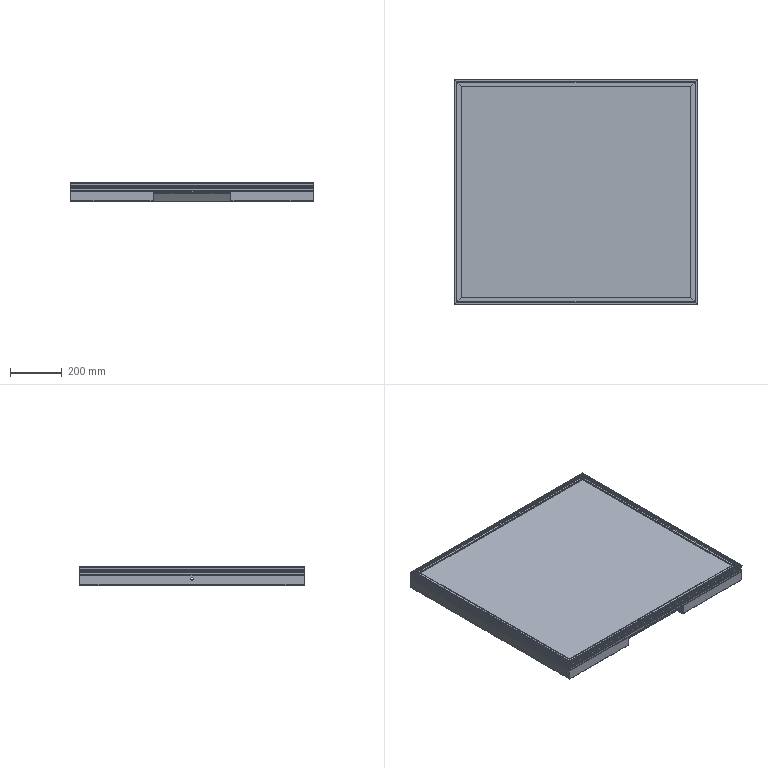Part | 9 solids | 894 faces | box 940 x 870 x 70 mm | volume 14410298 mm3 | plane 590 | cylinder 272 | spline 32 | commonest cylinder face diameters 7 x100 0.4 x67 2.4 x41 11 x28 2 x16 10 x12